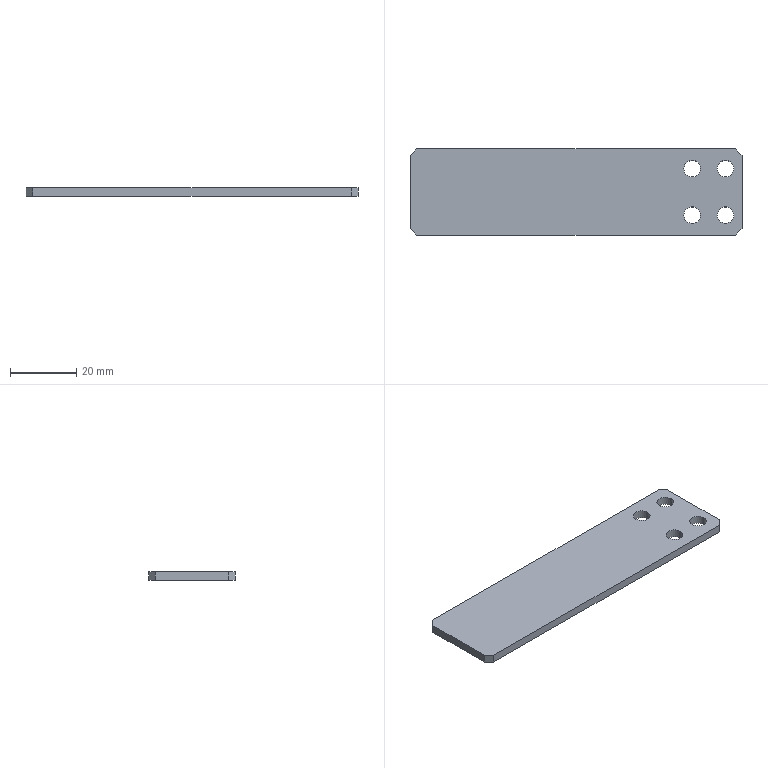Part | STEP file | 1 solid | 18 faces | box 100 x 26 x 2.5 mm | volume 6284 mm3 | plane 10 | cylinder 8 | commonest cylinder face diameters 5 x8
STEP:
#1=CARTESIAN_POINT('',(0.,0.,0.));
#2=DIRECTION('',(0.,0.,1.));
#3=DIRECTION('',(1.,0.,0.));
#4=AXIS2_PLACEMENT_3D('',#1,#2,#3);
#5=CARTESIAN_POINT('',(47.5,-7.,0.));
#6=VERTEX_POINT('',#5);
#7=CARTESIAN_POINT('',(47.5,-7.,2.5));
#8=VERTEX_POINT('',#7);
#9=CARTESIAN_POINT('',(47.5,-7.,0.));
#10=DIRECTION('',(0.,0.,1.));
#11=VECTOR('',#10,1.);
#12=LINE('',#9,#11);
#13=CARTESIAN_POINT('',(45.,-7.,0.));
#14=DIRECTION('',(0.,0.,1.));
#15=DIRECTION('',(1.,0.,0.));
#16=AXIS2_PLACEMENT_3D('',#13,#14,#15);
#17=CYLINDRICAL_SURFACE('',#16,2.5);
#18=CARTESIAN_POINT('',(6.283,0.));
#19=DIRECTION('',(0.,1.));
#20=VECTOR('',#19,1.);
#21=LINE('',#18,#20);
#22=(GEOMETRIC_REPRESENTATION_CONTEXT(2)PARAMETRIC_REPRESENTATION_CONTEXT()REPRESENTATION_CONTEXT('',''));
#23=DEFINITIONAL_REPRESENTATION('',(#21),#22);
#24=PCURVE('',#17,#23);
#25=CARTESIAN_POINT('',(45.,-7.,0.));
#26=DIRECTION('',(0.,0.,1.));
#27=DIRECTION('',(1.,0.,0.));
#28=AXIS2_PLACEMENT_3D('',#25,#26,#27);
#29=CYLINDRICAL_SURFACE('',#28,2.5);
#30=CARTESIAN_POINT('',(0.,0.));
#31=DIRECTION('',(0.,1.));
#32=VECTOR('',#31,1.);
#33=LINE('',#30,#32);
#34=(GEOMETRIC_REPRESENTATION_CONTEXT(2)PARAMETRIC_REPRESENTATION_CONTEXT()REPRESENTATION_CONTEXT('',''));
#35=DEFINITIONAL_REPRESENTATION('',(#33),#34);
#36=PCURVE('',#29,#35);
#37=SURFACE_CURVE('',#12,(#24,#36),.PCURVE_S1.);
#38=EDGE_CURVE('',#6,#8,#37,.T.);
#39=ORIENTED_EDGE('',*,*,#38,.T.);
#40=CARTESIAN_POINT('',(42.5,-7.,2.5));
#41=VERTEX_POINT('',#40);
#42=CARTESIAN_POINT('',(45.,-7.,2.5));
#43=DIRECTION('',(0.,0.,1.));
#44=DIRECTION('',(1.,0.,0.));
#45=AXIS2_PLACEMENT_3D('',#42,#43,#44);
#46=CIRCLE('',#45,2.5);
#47=CARTESIAN_POINT('',(0.,2.5));
#48=DIRECTION('',(1.,0.));
#49=VECTOR('',#48,1.);
#50=LINE('',#47,#49);
#51=(GEOMETRIC_REPRESENTATION_CONTEXT(2)PARAMETRIC_REPRESENTATION_CONTEXT()REPRESENTATION_CONTEXT('',''));
#52=DEFINITIONAL_REPRESENTATION('',(#50),#51);
#53=PCURVE('',#17,#52);
#54=CARTESIAN_POINT('',(-50.,-13.,2.5));
#55=DIRECTION('',(0.,0.,1.));
#56=DIRECTION('',(1.,0.,0.));
#57=AXIS2_PLACEMENT_3D('',#54,#55,#56);
#58=PLANE('',#57);
#59=CARTESIAN_POINT('',(95.,6.));
#60=DIRECTION('',(1.,0.));
#61=AXIS2_PLACEMENT_2D('',#59,#60);
#62=CIRCLE('',#61,2.5);
#63=(GEOMETRIC_REPRESENTATION_CONTEXT(2)PARAMETRIC_REPRESENTATION_CONTEXT()REPRESENTATION_CONTEXT('',''));
#64=DEFINITIONAL_REPRESENTATION('',(#62),#63);
#65=PCURVE('',#58,#64);
#66=SURFACE_CURVE('',#46,(#53,#65),.PCURVE_S1.);
#67=EDGE_CURVE('',#41,#8,#66,.T.);
#68=ORIENTED_EDGE('',*,*,#67,.F.);
#69=CARTESIAN_POINT('',(42.5,-7.,0.));
#70=VERTEX_POINT('',#69);
#71=CARTESIAN_POINT('',(42.5,-7.,0.));
#72=DIRECTION('',(0.,0.,1.));
#73=VECTOR('',#72,1.);
#74=LINE('',#71,#73);
#75=CARTESIAN_POINT('',(3.142,0.));
#76=DIRECTION('',(0.,1.));
#77=VECTOR('',#76,1.);
#78=LINE('',#75,#77);
#79=(GEOMETRIC_REPRESENTATION_CONTEXT(2)PARAMETRIC_REPRESENTATION_CONTEXT()REPRESENTATION_CONTEXT('',''));
#80=DEFINITIONAL_REPRESENTATION('',(#78),#79);
#81=PCURVE('',#17,#80);
#82=CARTESIAN_POINT('',(3.142,0.));
#83=DIRECTION('',(0.,1.));
#84=VECTOR('',#83,1.);
#85=LINE('',#82,#84);
#86=(GEOMETRIC_REPRESENTATION_CONTEXT(2)PARAMETRIC_REPRESENTATION_CONTEXT()REPRESENTATION_CONTEXT('',''));
#87=DEFINITIONAL_REPRESENTATION('',(#85),#86);
#88=PCURVE('',#29,#87);
#89=SURFACE_CURVE('',#74,(#81,#88),.PCURVE_S1.);
#90=EDGE_CURVE('',#70,#41,#89,.T.);
#91=ORIENTED_EDGE('',*,*,#90,.F.);
#92=CARTESIAN_POINT('',(45.,-7.,0.));
#93=DIRECTION('',(0.,0.,-1.));
#94=DIRECTION('',(1.,0.,0.));
#95=AXIS2_PLACEMENT_3D('',#92,#93,#94);
#96=CIRCLE('',#95,2.5);
#97=CARTESIAN_POINT('',(6.283,0.));
#98=DIRECTION('',(-1.,0.));
#99=VECTOR('',#98,1.);
#100=LINE('',#97,#99);
#101=(GEOMETRIC_REPRESENTATION_CONTEXT(2)PARAMETRIC_REPRESENTATION_CONTEXT()REPRESENTATION_CONTEXT('',''));
#102=DEFINITIONAL_REPRESENTATION('',(#100),#101);
#103=PCURVE('',#17,#102);
#104=CARTESIAN_POINT('',(-50.,-13.,0.));
#105=DIRECTION('',(0.,0.,1.));
#106=DIRECTION('',(1.,0.,0.));
#107=AXIS2_PLACEMENT_3D('',#104,#105,#106);
#108=PLANE('',#107);
#109=CARTESIAN_POINT('',(97.5,6.));
#110=CARTESIAN_POINT('',(97.5,1.67));
#111=CARTESIAN_POINT('',(93.75,3.835));
#112=CARTESIAN_POINT('',(90.,6.));
#113=CARTESIAN_POINT('',(93.75,8.165));
#114=CARTESIAN_POINT('',(97.5,10.33));
#115=CARTESIAN_POINT('',(97.5,6.));
#116=(BOUNDED_CURVE()B_SPLINE_CURVE(2,(#109,#110,#111,#112,#113,#114,#115),.UNSPECIFIED.,.T.,.F.)B_SPLINE_CURVE_WITH_KNOTS((1,2,2,2,2,1),(-2.094,0.,2.094,4.189,6.283,8.378),.UNSPECIFIED.)CURVE()GEOMETRIC_REPRESENTATION_ITEM()RATIONAL_B_SPLINE_CURVE((1.,0.5,1.,0.5,1.,0.5,1.))REPRESENTATION_ITEM(''));
#117=(GEOMETRIC_REPRESENTATION_CONTEXT(2)PARAMETRIC_REPRESENTATION_CONTEXT()REPRESENTATION_CONTEXT('',''));
#118=DEFINITIONAL_REPRESENTATION('',(#116),#117);
#119=PCURVE('',#108,#118);
#120=SURFACE_CURVE('',#96,(#103,#119),.PCURVE_S1.);
#121=EDGE_CURVE('',#6,#70,#120,.T.);
#122=ORIENTED_EDGE('',*,*,#121,.F.);
#123=EDGE_LOOP('',(#39,#68,#91,#122));
#124=FACE_BOUND('',#123,.F.);
#125=ADVANCED_FACE('',(#124),#17,.F.);
#126=CARTESIAN_POINT('',(47.5,7.,0.));
#127=VERTEX_POINT('',#126);
#128=CARTESIAN_POINT('',(47.5,7.,2.5));
#129=VERTEX_POINT('',#128);
#130=CARTESIAN_POINT('',(47.5,7.,0.));
#131=DIRECTION('',(0.,0.,1.));
#132=VECTOR('',#131,1.);
#133=LINE('',#130,#132);
#134=CARTESIAN_POINT('',(45.,7.,0.));
#135=DIRECTION('',(0.,0.,1.));
#136=DIRECTION('',(1.,0.,0.));
#137=AXIS2_PLACEMENT_3D('',#134,#135,#136);
#138=CYLINDRICAL_SURFACE('',#137,2.5);
#139=CARTESIAN_POINT('',(6.283,0.));
#140=DIRECTION('',(0.,1.));
#141=VECTOR('',#140,1.);
#142=LINE('',#139,#141);
#143=(GEOMETRIC_REPRESENTATION_CONTEXT(2)PARAMETRIC_REPRESENTATION_CONTEXT()REPRESENTATION_CONTEXT('',''));
#144=DEFINITIONAL_REPRESENTATION('',(#142),#143);
#145=PCURVE('',#138,#144);
#146=CARTESIAN_POINT('',(45.,7.,0.));
#147=DIRECTION('',(0.,0.,1.));
#148=DIRECTION('',(1.,0.,0.));
#149=AXIS2_PLACEMENT_3D('',#146,#147,#148);
#150=CYLINDRICAL_SURFACE('',#149,2.5);
#151=CARTESIAN_POINT('',(0.,0.));
#152=DIRECTION('',(0.,1.));
#153=VECTOR('',#152,1.);
#154=LINE('',#151,#153);
#155=(GEOMETRIC_REPRESENTATION_CONTEXT(2)PARAMETRIC_REPRESENTATION_CONTEXT()REPRESENTATION_CONTEXT('',''));
#156=DEFINITIONAL_REPRESENTATION('',(#154),#155);
#157=PCURVE('',#150,#156);
#158=SURFACE_CURVE('',#133,(#145,#157),.PCURVE_S1.);
#159=EDGE_CURVE('',#127,#129,#158,.T.);
#160=ORIENTED_EDGE('',*,*,#159,.T.);
#161=CARTESIAN_POINT('',(42.5,7.,2.5));
#162=VERTEX_POINT('',#161);
#163=CARTESIAN_POINT('',(45.,7.,2.5));
#164=DIRECTION('',(0.,0.,-1.));
#165=DIRECTION('',(1.,0.,0.));
#166=AXIS2_PLACEMENT_3D('',#163,#164,#165);
#167=CIRCLE('',#166,2.5);
#168=CARTESIAN_POINT('',(6.283,2.5));
#169=DIRECTION('',(-1.,0.));
#170=VECTOR('',#169,1.);
#171=LINE('',#168,#170);
#172=(GEOMETRIC_REPRESENTATION_CONTEXT(2)PARAMETRIC_REPRESENTATION_CONTEXT()REPRESENTATION_CONTEXT('',''));
#173=DEFINITIONAL_REPRESENTATION('',(#171),#172);
#174=PCURVE('',#138,#173);
#175=CARTESIAN_POINT('',(97.5,20.));
#176=CARTESIAN_POINT('',(97.5,15.67));
#177=CARTESIAN_POINT('',(93.75,17.835));
#178=CARTESIAN_POINT('',(90.,20.));
#179=CARTESIAN_POINT('',(93.75,22.165));
#180=CARTESIAN_POINT('',(97.5,24.33));
#181=CARTESIAN_POINT('',(97.5,20.));
#182=(BOUNDED_CURVE()B_SPLINE_CURVE(2,(#175,#176,#177,#178,#179,#180,#181),.UNSPECIFIED.,.T.,.F.)B_SPLINE_CURVE_WITH_KNOTS((1,2,2,2,2,1),(-2.094,0.,2.094,4.189,6.283,8.378),.UNSPECIFIED.)CURVE()GEOMETRIC_REPRESENTATION_ITEM()RATIONAL_B_SPLINE_CURVE((1.,0.5,1.,0.5,1.,0.5,1.))REPRESENTATION_ITEM(''));
#183=(GEOMETRIC_REPRESENTATION_CONTEXT(2)PARAMETRIC_REPRESENTATION_CONTEXT()REPRESENTATION_CONTEXT('',''));
#184=DEFINITIONAL_REPRESENTATION('',(#182),#183);
#185=PCURVE('',#58,#184);
#186=SURFACE_CURVE('',#167,(#174,#185),.PCURVE_S1.);
#187=EDGE_CURVE('',#129,#162,#186,.T.);
#188=ORIENTED_EDGE('',*,*,#187,.T.);
#189=CARTESIAN_POINT('',(42.5,7.,0.));
#190=VERTEX_POINT('',#189);
#191=CARTESIAN_POINT('',(42.5,7.,0.));
#192=DIRECTION('',(0.,0.,1.));
#193=VECTOR('',#192,1.);
#194=LINE('',#191,#193);
#195=CARTESIAN_POINT('',(3.142,0.));
#196=DIRECTION('',(0.,1.));
#197=VECTOR('',#196,1.);
#198=LINE('',#195,#197);
#199=(GEOMETRIC_REPRESENTATION_CONTEXT(2)PARAMETRIC_REPRESENTATION_CONTEXT()REPRESENTATION_CONTEXT('',''));
#200=DEFINITIONAL_REPRESENTATION('',(#198),#199);
#201=PCURVE('',#138,#200);
#202=CARTESIAN_POINT('',(3.142,0.));
#203=DIRECTION('',(0.,1.));
#204=VECTOR('',#203,1.);
#205=LINE('',#202,#204);
#206=(GEOMETRIC_REPRESENTATION_CONTEXT(2)PARAMETRIC_REPRESENTATION_CONTEXT()REPRESENTATION_CONTEXT('',''));
#207=DEFINITIONAL_REPRESENTATION('',(#205),#206);
#208=PCURVE('',#150,#207);
#209=SURFACE_CURVE('',#194,(#201,#208),.PCURVE_S1.);
#210=EDGE_CURVE('',#190,#162,#209,.T.);
#211=ORIENTED_EDGE('',*,*,#210,.F.);
#212=CARTESIAN_POINT('',(45.,7.,0.));
#213=DIRECTION('',(0.,0.,-1.));
#214=DIRECTION('',(1.,0.,0.));
#215=AXIS2_PLACEMENT_3D('',#212,#213,#214);
#216=CIRCLE('',#215,2.5);
#217=CARTESIAN_POINT('',(6.283,0.));
#218=DIRECTION('',(-1.,0.));
#219=VECTOR('',#218,1.);
#220=LINE('',#217,#219);
#221=(GEOMETRIC_REPRESENTATION_CONTEXT(2)PARAMETRIC_REPRESENTATION_CONTEXT()REPRESENTATION_CONTEXT('',''));
#222=DEFINITIONAL_REPRESENTATION('',(#220),#221);
#223=PCURVE('',#138,#222);
#224=CARTESIAN_POINT('',(97.5,20.));
#225=CARTESIAN_POINT('',(97.5,15.67));
#226=CARTESIAN_POINT('',(93.75,17.835));
#227=CARTESIAN_POINT('',(90.,20.));
#228=CARTESIAN_POINT('',(93.75,22.165));
#229=CARTESIAN_POINT('',(97.5,24.33));
#230=CARTESIAN_POINT('',(97.5,20.));
#231=(BOUNDED_CURVE()B_SPLINE_CURVE(2,(#224,#225,#226,#227,#228,#229,#230),.UNSPECIFIED.,.T.,.F.)B_SPLINE_CURVE_WITH_KNOTS((1,2,2,2,2,1),(-2.094,0.,2.094,4.189,6.283,8.378),.UNSPECIFIED.)CURVE()GEOMETRIC_REPRESENTATION_ITEM()RATIONAL_B_SPLINE_CURVE((1.,0.5,1.,0.5,1.,0.5,1.))REPRESENTATION_ITEM(''));
#232=(GEOMETRIC_REPRESENTATION_CONTEXT(2)PARAMETRIC_REPRESENTATION_CONTEXT()REPRESENTATION_CONTEXT('',''));
#233=DEFINITIONAL_REPRESENTATION('',(#231),#232);
#234=PCURVE('',#108,#233);
#235=SURFACE_CURVE('',#216,(#223,#234),.PCURVE_S1.);
#236=EDGE_CURVE('',#127,#190,#235,.T.);
#237=ORIENTED_EDGE('',*,*,#236,.F.);
#238=EDGE_LOOP('',(#160,#188,#211,#237));
#239=FACE_BOUND('',#238,.F.);
#240=ADVANCED_FACE('',(#239),#138,.F.);
#241=CARTESIAN_POINT('',(37.5,7.,0.));
#242=VERTEX_POINT('',#241);
#243=CARTESIAN_POINT('',(37.5,7.,2.5));
#244=VERTEX_POINT('',#243);
#245=CARTESIAN_POINT('',(37.5,7.,0.));
#246=DIRECTION('',(0.,0.,1.));
#247=VECTOR('',#246,1.);
#248=LINE('',#245,#247);
#249=CARTESIAN_POINT('',(35.,7.,0.));
#250=DIRECTION('',(0.,0.,1.));
#251=DIRECTION('',(1.,0.,0.));
#252=AXIS2_PLACEMENT_3D('',#249,#250,#251);
#253=CYLINDRICAL_SURFACE('',#252,2.5);
#254=CARTESIAN_POINT('',(6.283,0.));
#255=DIRECTION('',(0.,1.));
#256=VECTOR('',#255,1.);
#257=LINE('',#254,#256);
#258=(GEOMETRIC_REPRESENTATION_CONTEXT(2)PARAMETRIC_REPRESENTATION_CONTEXT()REPRESENTATION_CONTEXT('',''));
#259=DEFINITIONAL_REPRESENTATION('',(#257),#258);
#260=PCURVE('',#253,#259);
#261=CARTESIAN_POINT('',(35.,7.,0.));
#262=DIRECTION('',(0.,0.,1.));
#263=DIRECTION('',(1.,0.,0.));
#264=AXIS2_PLACEMENT_3D('',#261,#262,#263);
#265=CYLINDRICAL_SURFACE('',#264,2.5);
#266=CARTESIAN_POINT('',(0.,0.));
#267=DIRECTION('',(0.,1.));
#268=VECTOR('',#267,1.);
#269=LINE('',#266,#268);
#270=(GEOMETRIC_REPRESENTATION_CONTEXT(2)PARAMETRIC_REPRESENTATION_CONTEXT()REPRESENTATION_CONTEXT('',''));
#271=DEFINITIONAL_REPRESENTATION('',(#269),#270);
#272=PCURVE('',#265,#271);
#273=SURFACE_CURVE('',#248,(#260,#272),.PCURVE_S1.);
#274=EDGE_CURVE('',#242,#244,#273,.T.);
#275=ORIENTED_EDGE('',*,*,#274,.T.);
#276=CARTESIAN_POINT('',(32.5,7.,2.5));
#277=VERTEX_POINT('',#276);
#278=CARTESIAN_POINT('',(35.,7.,2.5));
#279=DIRECTION('',(0.,0.,-1.));
#280=DIRECTION('',(1.,0.,0.));
#281=AXIS2_PLACEMENT_3D('',#278,#279,#280);
#282=CIRCLE('',#281,2.5);
#283=CARTESIAN_POINT('',(6.283,2.5));
#284=DIRECTION('',(-1.,0.));
#285=VECTOR('',#284,1.);
#286=LINE('',#283,#285);
#287=(GEOMETRIC_REPRESENTATION_CONTEXT(2)PARAMETRIC_REPRESENTATION_CONTEXT()REPRESENTATION_CONTEXT('',''));
#288=DEFINITIONAL_REPRESENTATION('',(#286),#287);
#289=PCURVE('',#253,#288);
#290=CARTESIAN_POINT('',(87.5,20.));
#291=CARTESIAN_POINT('',(87.5,15.67));
#292=CARTESIAN_POINT('',(83.75,17.835));
#293=CARTESIAN_POINT('',(80.,20.));
#294=CARTESIAN_POINT('',(83.75,22.165));
#295=CARTESIAN_POINT('',(87.5,24.33));
#296=CARTESIAN_POINT('',(87.5,20.));
#297=(BOUNDED_CURVE()B_SPLINE_CURVE(2,(#290,#291,#292,#293,#294,#295,#296),.UNSPECIFIED.,.T.,.F.)B_SPLINE_CURVE_WITH_KNOTS((1,2,2,2,2,1),(-2.094,0.,2.094,4.189,6.283,8.378),.UNSPECIFIED.)CURVE()GEOMETRIC_REPRESENTATION_ITEM()RATIONAL_B_SPLINE_CURVE((1.,0.5,1.,0.5,1.,0.5,1.))REPRESENTATION_ITEM(''));
#298=(GEOMETRIC_REPRESENTATION_CONTEXT(2)PARAMETRIC_REPRESENTATION_CONTEXT()REPRESENTATION_CONTEXT('',''));
#299=DEFINITIONAL_REPRESENTATION('',(#297),#298);
#300=PCURVE('',#58,#299);
#301=SURFACE_CURVE('',#282,(#289,#300),.PCURVE_S1.);
#302=EDGE_CURVE('',#244,#277,#301,.T.);
#303=ORIENTED_EDGE('',*,*,#302,.T.);
#304=CARTESIAN_POINT('',(32.5,7.,0.));
#305=VERTEX_POINT('',#304);
#306=CARTESIAN_POINT('',(32.5,7.,0.));
#307=DIRECTION('',(0.,0.,1.));
#308=VECTOR('',#307,1.);
#309=LINE('',#306,#308);
#310=CARTESIAN_POINT('',(3.142,0.));
#311=DIRECTION('',(0.,1.));
#312=VECTOR('',#311,1.);
#313=LINE('',#310,#312);
#314=(GEOMETRIC_REPRESENTATION_CONTEXT(2)PARAMETRIC_REPRESENTATION_CONTEXT()REPRESENTATION_CONTEXT('',''));
#315=DEFINITIONAL_REPRESENTATION('',(#313),#314);
#316=PCURVE('',#253,#315);
#317=CARTESIAN_POINT('',(3.142,0.));
#318=DIRECTION('',(0.,1.));
#319=VECTOR('',#318,1.);
#320=LINE('',#317,#319);
#321=(GEOMETRIC_REPRESENTATION_CONTEXT(2)PARAMETRIC_REPRESENTATION_CONTEXT()REPRESENTATION_CONTEXT('',''));
#322=DEFINITIONAL_REPRESENTATION('',(#320),#321);
#323=PCURVE('',#265,#322);
#324=SURFACE_CURVE('',#309,(#316,#323),.PCURVE_S1.);
#325=EDGE_CURVE('',#305,#277,#324,.T.);
#326=ORIENTED_EDGE('',*,*,#325,.F.);
#327=CARTESIAN_POINT('',(35.,7.,0.));
#328=DIRECTION('',(0.,0.,-1.));
#329=DIRECTION('',(1.,0.,0.));
#330=AXIS2_PLACEMENT_3D('',#327,#328,#329);
#331=CIRCLE('',#330,2.5);
#332=CARTESIAN_POINT('',(6.283,0.));
#333=DIRECTION('',(-1.,0.));
#334=VECTOR('',#333,1.);
#335=LINE('',#332,#334);
#336=(GEOMETRIC_REPRESENTATION_CONTEXT(2)PARAMETRIC_REPRESENTATION_CONTEXT()REPRESENTATION_CONTEXT('',''));
#337=DEFINITIONAL_REPRESENTATION('',(#335),#336);
#338=PCURVE('',#253,#337);
#339=CARTESIAN_POINT('',(87.5,20.));
#340=CARTESIAN_POINT('',(87.5,15.67));
#341=CARTESIAN_POINT('',(83.75,17.835));
#342=CARTESIAN_POINT('',(80.,20.));
#343=CARTESIAN_POINT('',(83.75,22.165));
#344=CARTESIAN_POINT('',(87.5,24.33));
#345=CARTESIAN_POINT('',(87.5,20.));
#346=(BOUNDED_CURVE()B_SPLINE_CURVE(2,(#339,#340,#341,#342,#343,#344,#345),.UNSPECIFIED.,.T.,.F.)B_SPLINE_CURVE_WITH_KNOTS((1,2,2,2,2,1),(-2.094,0.,2.094,4.189,6.283,8.378),.UNSPECIFIED.)CURVE()GEOMETRIC_REPRESENTATION_ITEM()RATIONAL_B_SPLINE_CURVE((1.,0.5,1.,0.5,1.,0.5,1.))REPRESENTATION_ITEM(''));
#347=(GEOMETRIC_REPRESENTATION_CONTEXT(2)PARAMETRIC_REPRESENTATION_CONTEXT()REPRESENTATION_CONTEXT('',''));
#348=DEFINITIONAL_REPRESENTATION('',(#346),#347);
#349=PCURVE('',#108,#348);
#350=SURFACE_CURVE('',#331,(#338,#349),.PCURVE_S1.);
#351=EDGE_CURVE('',#242,#305,#350,.T.);
#352=ORIENTED_EDGE('',*,*,#351,.F.);
#353=EDGE_LOOP('',(#275,#303,#326,#352));
#354=FACE_BOUND('',#353,.F.);
#355=ADVANCED_FACE('',(#354),#253,.F.);
#356=CARTESIAN_POINT('',(37.5,-7.,0.));
#357=VERTEX_POINT('',#356);
#358=CARTESIAN_POINT('',(37.5,-7.,2.5));
#359=VERTEX_POINT('',#358);
#360=CARTESIAN_POINT('',(37.5,-7.,0.));
#361=DIRECTION('',(0.,0.,1.));
#362=VECTOR('',#361,1.);
#363=LINE('',#360,#362);
#364=CARTESIAN_POINT('',(35.,-7.,0.));
#365=DIRECTION('',(0.,0.,1.));
#366=DIRECTION('',(1.,0.,0.));
#367=AXIS2_PLACEMENT_3D('',#364,#365,#366);
#368=CYLINDRICAL_SURFACE('',#367,2.5);
#369=CARTESIAN_POINT('',(6.283,0.));
#370=DIRECTION('',(0.,1.));
#371=VECTOR('',#370,1.);
#372=LINE('',#369,#371);
#373=(GEOMETRIC_REPRESENTATION_CONTEXT(2)PARAMETRIC_REPRESENTATION_CONTEXT()REPRESENTATION_CONTEXT('',''));
#374=DEFINITIONAL_REPRESENTATION('',(#372),#373);
#375=PCURVE('',#368,#374);
#376=CARTESIAN_POINT('',(35.,-7.,0.));
#377=DIRECTION('',(0.,0.,1.));
#378=DIRECTION('',(1.,0.,0.));
#379=AXIS2_PLACEMENT_3D('',#376,#377,#378);
#380=CYLINDRICAL_SURFACE('',#379,2.5);
#381=CARTESIAN_POINT('',(0.,0.));
#382=DIRECTION('',(0.,1.));
#383=VECTOR('',#382,1.);
#384=LINE('',#381,#383);
#385=(GEOMETRIC_REPRESENTATION_CONTEXT(2)PARAMETRIC_REPRESENTATION_CONTEXT()REPRESENTATION_CONTEXT('',''));
#386=DEFINITIONAL_REPRESENTATION('',(#384),#385);
#387=PCURVE('',#380,#386);
#388=SURFACE_CURVE('',#363,(#375,#387),.PCURVE_S1.);
#389=EDGE_CURVE('',#357,#359,#388,.T.);
#390=ORIENTED_EDGE('',*,*,#389,.T.);
#391=CARTESIAN_POINT('',(32.5,-7.,2.5));
#392=VERTEX_POINT('',#391);
#393=CARTESIAN_POINT('',(35.,-7.,2.5));
#394=DIRECTION('',(0.,0.,-1.));
#395=DIRECTION('',(1.,0.,0.));
#396=AXIS2_PLACEMENT_3D('',#393,#394,#395);
#397=CIRCLE('',#396,2.5);
#398=CARTESIAN_POINT('',(6.283,2.5));
#399=DIRECTION('',(-1.,0.));
#400=VECTOR('',#399,1.);
#401=LINE('',#398,#400);
#402=(GEOMETRIC_REPRESENTATION_CONTEXT(2)PARAMETRIC_REPRESENTATION_CONTEXT()REPRESENTATION_CONTEXT('',''));
#403=DEFINITIONAL_REPRESENTATION('',(#401),#402);
#404=PCURVE('',#368,#403);
#405=CARTESIAN_POINT('',(87.5,6.));
#406=CARTESIAN_POINT('',(87.5,1.67));
#407=CARTESIAN_POINT('',(83.75,3.835));
#408=CARTESIAN_POINT('',(80.,6.));
#409=CARTESIAN_POINT('',(83.75,8.165));
#410=CARTESIAN_POINT('',(87.5,10.33));
#411=CARTESIAN_POINT('',(87.5,6.));
#412=(BOUNDED_CURVE()B_SPLINE_CURVE(2,(#405,#406,#407,#408,#409,#410,#411),.UNSPECIFIED.,.T.,.F.)B_SPLINE_CURVE_WITH_KNOTS((1,2,2,2,2,1),(-2.094,0.,2.094,4.189,6.283,8.378),.UNSPECIFIED.)CURVE()GEOMETRIC_REPRESENTATION_ITEM()RATIONAL_B_SPLINE_CURVE((1.,0.5,1.,0.5,1.,0.5,1.))REPRESENTATION_ITEM(''));
#413=(GEOMETRIC_REPRESENTATION_CONTEXT(2)PARAMETRIC_REPRESENTATION_CONTEXT()REPRESENTATION_CONTEXT('',''));
#414=DEFINITIONAL_REPRESENTATION('',(#412),#413);
#415=PCURVE('',#58,#414);
#416=SURFACE_CURVE('',#397,(#404,#415),.PCURVE_S1.);
#417=EDGE_CURVE('',#359,#392,#416,.T.);
#418=ORIENTED_EDGE('',*,*,#417,.T.);
#419=CARTESIAN_POINT('',(32.5,-7.,0.));
#420=VERTEX_POINT('',#419);
#421=CARTESIAN_POINT('',(32.5,-7.,0.));
#422=DIRECTION('',(0.,0.,1.));
#423=VECTOR('',#422,1.);
#424=LINE('',#421,#423);
#425=CARTESIAN_POINT('',(3.142,0.));
#426=DIRECTION('',(0.,1.));
#427=VECTOR('',#426,1.);
#428=LINE('',#425,#427);
#429=(GEOMETRIC_REPRESENTATION_CONTEXT(2)PARAMETRIC_REPRESENTATION_CONTEXT()REPRESENTATION_CONTEXT('',''));
#430=DEFINITIONAL_REPRESENTATION('',(#428),#429);
#431=PCURVE('',#368,#430);
#432=CARTESIAN_POINT('',(3.142,0.));
#433=DIRECTION('',(0.,1.));
#434=VECTOR('',#433,1.);
#435=LINE('',#432,#434);
#436=(GEOMETRIC_REPRESENTATION_CONTEXT(2)PARAMETRIC_REPRESENTATION_CONTEXT()REPRESENTATION_CONTEXT('',''));
#437=DEFINITIONAL_REPRESENTATION('',(#435),#436);
#438=PCURVE('',#380,#437);
#439=SURFACE_CURVE('',#424,(#431,#438),.PCURVE_S1.);
#440=EDGE_CURVE('',#420,#392,#439,.T.);
#441=ORIENTED_EDGE('',*,*,#440,.F.);
#442=CARTESIAN_POINT('',(35.,-7.,0.));
#443=DIRECTION('',(0.,0.,-1.));
#444=DIRECTION('',(1.,0.,0.));
#445=AXIS2_PLACEMENT_3D('',#442,#443,#444);
#446=CIRCLE('',#445,2.5);
#447=CARTESIAN_POINT('',(6.283,0.));
#448=DIRECTION('',(-1.,0.));
#449=VECTOR('',#448,1.);
#450=LINE('',#447,#449);
#451=(GEOMETRIC_REPRESENTATION_CONTEXT(2)PARAMETRIC_REPRESENTATION_CONTEXT()REPRESENTATION_CONTEXT('',''));
#452=DEFINITIONAL_REPRESENTATION('',(#450),#451);
#453=PCURVE('',#368,#452);
#454=CARTESIAN_POINT('',(87.5,6.));
#455=CARTESIAN_POINT('',(87.5,1.67));
#456=CARTESIAN_POINT('',(83.75,3.835));
#457=CARTESIAN_POINT('',(80.,6.));
#458=CARTESIAN_POINT('',(83.75,8.165));
#459=CARTESIAN_POINT('',(87.5,10.33));
#460=CARTESIAN_POINT('',(87.5,6.));
#461=(BOUNDED_CURVE()B_SPLINE_CURVE(2,(#454,#455,#456,#457,#458,#459,#460),.UNSPECIFIED.,.T.,.F.)B_SPLINE_CURVE_WITH_KNOTS((1,2,2,2,2,1),(-2.094,0.,2.094,4.189,6.283,8.378),.UNSPECIFIED.)CURVE()GEOMETRIC_REPRESENTATION_ITEM()RATIONAL_B_SPLINE_CURVE((1.,0.5,1.,0.5,1.,0.5,1.))REPRESENTATION_ITEM(''));
#462=(GEOMETRIC_REPRESENTATION_CONTEXT(2)PARAMETRIC_REPRESENTATION_CONTEXT()REPRESENTATION_CONTEXT('',''));
#463=DEFINITIONAL_REPRESENTATION('',(#461),#462);
#464=PCURVE('',#108,#463);
#465=SURFACE_CURVE('',#446,(#453,#464),.PCURVE_S1.);
#466=EDGE_CURVE('',#357,#420,#465,.T.);
#467=ORIENTED_EDGE('',*,*,#466,.F.);
#468=EDGE_LOOP('',(#390,#418,#441,#467));
#469=FACE_BOUND('',#468,.F.);
#470=ADVANCED_FACE('',(#469),#368,.F.);
#471=CARTESIAN_POINT('',(45.,-7.,2.5));
#472=DIRECTION('',(0.,0.,1.));
#473=DIRECTION('',(1.,0.,0.));
#474=AXIS2_PLACEMENT_3D('',#471,#472,#473);
#475=CIRCLE('',#474,2.5);
#476=CARTESIAN_POINT('',(0.,2.5));
#477=DIRECTION('',(1.,0.));
#478=VECTOR('',#477,1.);
#479=LINE('',#476,#478);
#480=(GEOMETRIC_REPRESENTATION_CONTEXT(2)PARAMETRIC_REPRESENTATION_CONTEXT()REPRESENTATION_CONTEXT('',''));
#481=DEFINITIONAL_REPRESENTATION('',(#479),#480);
#482=PCURVE('',#29,#481);
#483=CARTESIAN_POINT('',(95.,6.));
#484=DIRECTION('',(1.,0.));
#485=AXIS2_PLACEMENT_2D('',#483,#484);
#486=CIRCLE('',#485,2.5);
#487=(GEOMETRIC_REPRESENTATION_CONTEXT(2)PARAMETRIC_REPRESENTATION_CONTEXT()REPRESENTATION_CONTEXT('',''));
#488=DEFINITIONAL_REPRESENTATION('',(#486),#487);
#489=PCURVE('',#58,#488);
#490=SURFACE_CURVE('',#475,(#482,#489),.PCURVE_S1.);
#491=EDGE_CURVE('',#8,#41,#490,.T.);
#492=ORIENTED_EDGE('',*,*,#491,.F.);
#493=ORIENTED_EDGE('',*,*,#38,.F.);
#494=CARTESIAN_POINT('',(45.,-7.,0.));
#495=DIRECTION('',(0.,0.,-1.));
#496=DIRECTION('',(1.,0.,0.));
#497=AXIS2_PLACEMENT_3D('',#494,#495,#496);
#498=CIRCLE('',#497,2.5);
#499=CARTESIAN_POINT('',(6.283,0.));
#500=DIRECTION('',(-1.,0.));
#501=VECTOR('',#500,1.);
#502=LINE('',#499,#501);
#503=(GEOMETRIC_REPRESENTATION_CONTEXT(2)PARAMETRIC_REPRESENTATION_CONTEXT()REPRESENTATION_CONTEXT('',''));
#504=DEFINITIONAL_REPRESENTATION('',(#502),#503);
#505=PCURVE('',#29,#504);
#506=CARTESIAN_POINT('',(97.5,6.));
#507=CARTESIAN_POINT('',(97.5,1.67));
#508=CARTESIAN_POINT('',(93.75,3.835));
#509=CARTESIAN_POINT('',(90.,6.));
#510=CARTESIAN_POINT('',(93.75,8.165));
#511=CARTESIAN_POINT('',(97.5,10.33));
#512=CARTESIAN_POINT('',(97.5,6.));
#513=(BOUNDED_CURVE()B_SPLINE_CURVE(2,(#506,#507,#508,#509,#510,#511,#512),.UNSPECIFIED.,.T.,.F.)B_SPLINE_CURVE_WITH_KNOTS((1,2,2,2,2,1),(-2.094,0.,2.094,4.189,6.283,8.378),.UNSPECIFIED.)CURVE()GEOMETRIC_REPRESENTATION_ITEM()RATIONAL_B_SPLINE_CURVE((1.,0.5,1.,0.5,1.,0.5,1.))REPRESENTATION_ITEM(''));
#514=(GEOMETRIC_REPRESENTATION_CONTEXT(2)PARAMETRIC_REPRESENTATION_CONTEXT()REPRESENTATION_CONTEXT('',''));
#515=DEFINITIONAL_REPRESENTATION('',(#513),#514);
#516=PCURVE('',#108,#515);
#517=SURFACE_CURVE('',#498,(#505,#516),.PCURVE_S1.);
#518=EDGE_CURVE('',#70,#6,#517,.T.);
#519=ORIENTED_EDGE('',*,*,#518,.F.);
#520=ORIENTED_EDGE('',*,*,#90,.T.);
#521=EDGE_LOOP('',(#492,#493,#519,#520));
#522=FACE_BOUND('',#521,.F.);
#523=ADVANCED_FACE('',(#522),#29,.F.);
#524=ORIENTED_EDGE('',*,*,#187,.T.);
#525=CARTESIAN_POINT('',(45.,7.,2.5));
#526=DIRECTION('',(0.,0.,-1.));
#527=DIRECTION('',(1.,0.,0.));
#528=AXIS2_PLACEMENT_3D('',#525,#526,#527);
#529=CIRCLE('',#528,2.5);
#530=CARTESIAN_POINT('',(97.5,20.));
#531=CARTESIAN_POINT('',(97.5,15.67));
#532=CARTESIAN_POINT('',(93.75,17.835));
#533=CARTESIAN_POINT('',(90.,20.));
#534=CARTESIAN_POINT('',(93.75,22.165));
#535=CARTESIAN_POINT('',(97.5,24.33));
#536=CARTESIAN_POINT('',(97.5,20.));
#537=(BOUNDED_CURVE()B_SPLINE_CURVE(2,(#530,#531,#532,#533,#534,#535,#536),.UNSPECIFIED.,.T.,.F.)B_SPLINE_CURVE_WITH_KNOTS((1,2,2,2,2,1),(-2.094,0.,2.094,4.189,6.283,8.378),.UNSPECIFIED.)CURVE()GEOMETRIC_REPRESENTATION_ITEM()RATIONAL_B_SPLINE_CURVE((1.,0.5,1.,0.5,1.,0.5,1.))REPRESENTATION_ITEM(''));
#538=(GEOMETRIC_REPRESENTATION_CONTEXT(2)PARAMETRIC_REPRESENTATION_CONTEXT()REPRESENTATION_CONTEXT('',''));
#539=DEFINITIONAL_REPRESENTATION('',(#537),#538);
#540=PCURVE('',#58,#539);
#541=CARTESIAN_POINT('',(6.283,2.5));
#542=DIRECTION('',(-1.,0.));
#543=VECTOR('',#542,1.);
#544=LINE('',#541,#543);
#545=(GEOMETRIC_REPRESENTATION_CONTEXT(2)PARAMETRIC_REPRESENTATION_CONTEXT()REPRESENTATION_CONTEXT('',''));
#546=DEFINITIONAL_REPRESENTATION('',(#544),#545);
#547=PCURVE('',#150,#546);
#548=SURFACE_CURVE('',#529,(#540,#547),.PCURVE_S1.);
#549=EDGE_CURVE('',#162,#129,#548,.T.);
#550=ORIENTED_EDGE('',*,*,#549,.T.);
#551=EDGE_LOOP('',(#524,#550));
#552=FACE_BOUND('',#551,.T.);
#553=ORIENTED_EDGE('',*,*,#302,.T.);
#554=CARTESIAN_POINT('',(35.,7.,2.5));
#555=DIRECTION('',(0.,0.,-1.));
#556=DIRECTION('',(1.,0.,0.));
#557=AXIS2_PLACEMENT_3D('',#554,#555,#556);
#558=CIRCLE('',#557,2.5);
#559=CARTESIAN_POINT('',(87.5,20.));
#560=CARTESIAN_POINT('',(87.5,15.67));
#561=CARTESIAN_POINT('',(83.75,17.835));
#562=CARTESIAN_POINT('',(80.,20.));
#563=CARTESIAN_POINT('',(83.75,22.165));
#564=CARTESIAN_POINT('',(87.5,24.33));
#565=CARTESIAN_POINT('',(87.5,20.));
#566=(BOUNDED_CURVE()B_SPLINE_CURVE(2,(#559,#560,#561,#562,#563,#564,#565),.UNSPECIFIED.,.T.,.F.)B_SPLINE_CURVE_WITH_KNOTS((1,2,2,2,2,1),(-2.094,0.,2.094,4.189,6.283,8.378),.UNSPECIFIED.)CURVE()GEOMETRIC_REPRESENTATION_ITEM()RATIONAL_B_SPLINE_CURVE((1.,0.5,1.,0.5,1.,0.5,1.))REPRESENTATION_ITEM(''));
#567=(GEOMETRIC_REPRESENTATION_CONTEXT(2)PARAMETRIC_REPRESENTATION_CONTEXT()REPRESENTATION_CONTEXT('',''));
#568=DEFINITIONAL_REPRESENTATION('',(#566),#567);
#569=PCURVE('',#58,#568);
#570=CARTESIAN_POINT('',(6.283,2.5));
#571=DIRECTION('',(-1.,0.));
#572=VECTOR('',#571,1.);
#573=LINE('',#570,#572);
#574=(GEOMETRIC_REPRESENTATION_CONTEXT(2)PARAMETRIC_REPRESENTATION_CONTEXT()REPRESENTATION_CONTEXT('',''));
#575=DEFINITIONAL_REPRESENTATION('',(#573),#574);
#576=PCURVE('',#265,#575);
#577=SURFACE_CURVE('',#558,(#569,#576),.PCURVE_S1.);
#578=EDGE_CURVE('',#277,#244,#577,.T.);
#579=ORIENTED_EDGE('',*,*,#578,.T.);
#580=EDGE_LOOP('',(#553,#579));
#581=FACE_BOUND('',#580,.T.);
#582=ORIENTED_EDGE('',*,*,#417,.T.);
#583=CARTESIAN_POINT('',(35.,-7.,2.5));
#584=DIRECTION('',(0.,0.,-1.));
#585=DIRECTION('',(1.,0.,0.));
#586=AXIS2_PLACEMENT_3D('',#583,#584,#585);
#587=CIRCLE('',#586,2.5);
#588=CARTESIAN_POINT('',(87.5,6.));
#589=CARTESIAN_POINT('',(87.5,1.67));
#590=CARTESIAN_POINT('',(83.75,3.835));
#591=CARTESIAN_POINT('',(80.,6.));
#592=CARTESIAN_POINT('',(83.75,8.165));
#593=CARTESIAN_POINT('',(87.5,10.33));
#594=CARTESIAN_POINT('',(87.5,6.));
#595=(BOUNDED_CURVE()B_SPLINE_CURVE(2,(#588,#589,#590,#591,#592,#593,#594),.UNSPECIFIED.,.T.,.F.)B_SPLINE_CURVE_WITH_KNOTS((1,2,2,2,2,1),(-2.094,0.,2.094,4.189,6.283,8.378),.UNSPECIFIED.)CURVE()GEOMETRIC_REPRESENTATION_ITEM()RATIONAL_B_SPLINE_CURVE((1.,0.5,1.,0.5,1.,0.5,1.))REPRESENTATION_ITEM(''));
#596=(GEOMETRIC_REPRESENTATION_CONTEXT(2)PARAMETRIC_REPRESENTATION_CONTEXT()REPRESENTATION_CONTEXT('',''));
#597=DEFINITIONAL_REPRESENTATION('',(#595),#596);
#598=PCURVE('',#58,#597);
#599=CARTESIAN_POINT('',(6.283,2.5));
#600=DIRECTION('',(-1.,0.));
#601=VECTOR('',#600,1.);
#602=LINE('',#599,#601);
#603=(GEOMETRIC_REPRESENTATION_CONTEXT(2)PARAMETRIC_REPRESENTATION_CONTEXT()REPRESENTATION_CONTEXT('',''));
#604=DEFINITIONAL_REPRESENTATION('',(#602),#603);
#605=PCURVE('',#380,#604);
#606=SURFACE_CURVE('',#587,(#598,#605),.PCURVE_S1.);
#607=EDGE_CURVE('',#392,#359,#606,.T.);
#608=ORIENTED_EDGE('',*,*,#607,.T.);
#609=EDGE_LOOP('',(#582,#608));
#610=FACE_BOUND('',#609,.T.);
#611=ORIENTED_EDGE('',*,*,#491,.F.);
#612=ORIENTED_EDGE('',*,*,#67,.F.);
#613=EDGE_LOOP('',(#611,#612));
#614=FACE_BOUND('',#613,.T.);
#615=CARTESIAN_POINT('',(50.,-11.,2.5));
#616=VERTEX_POINT('',#615);
#617=CARTESIAN_POINT('',(50.,11.,2.5));
#618=VERTEX_POINT('',#617);
#619=CARTESIAN_POINT('',(50.,0.,2.5));
#620=DIRECTION('',(0.,1.,0.));
#621=VECTOR('',#620,1.);
#622=LINE('',#619,#621);
#623=CARTESIAN_POINT('',(100.,13.));
#624=DIRECTION('',(0.,1.));
#625=VECTOR('',#624,1.);
#626=LINE('',#623,#625);
#627=(GEOMETRIC_REPRESENTATION_CONTEXT(2)PARAMETRIC_REPRESENTATION_CONTEXT()REPRESENTATION_CONTEXT('',''));
#628=DEFINITIONAL_REPRESENTATION('',(#626),#627);
#629=PCURVE('',#58,#628);
#630=CARTESIAN_POINT('',(50.,-11.,0.));
#631=DIRECTION('',(-1.,0.,0.));
#632=DIRECTION('',(0.,0.,1.));
#633=AXIS2_PLACEMENT_3D('',#630,#631,#632);
#634=PLANE('',#633);
#635=CARTESIAN_POINT('',(2.5,11.));
#636=DIRECTION('',(0.,1.));
#637=VECTOR('',#636,1.);
#638=LINE('',#635,#637);
#639=(GEOMETRIC_REPRESENTATION_CONTEXT(2)PARAMETRIC_REPRESENTATION_CONTEXT()REPRESENTATION_CONTEXT('',''));
#640=DEFINITIONAL_REPRESENTATION('',(#638),#639);
#641=PCURVE('',#634,#640);
#642=SURFACE_CURVE('',#622,(#629,#641),.PCURVE_S1.);
#643=EDGE_CURVE('',#616,#618,#642,.T.);
#644=ORIENTED_EDGE('',*,*,#643,.T.);
#645=CARTESIAN_POINT('',(48.,13.,2.5));
#646=VERTEX_POINT('',#645);
#647=CARTESIAN_POINT('',(50.,11.,2.5));
#648=DIRECTION('',(-0.7071,0.7071,0.));
#649=VECTOR('',#648,1.);
#650=LINE('',#647,#649);
#651=CARTESIAN_POINT('',(100.,24.));
#652=DIRECTION('',(-0.7071,0.7071));
#653=VECTOR('',#652,1.);
#654=LINE('',#651,#653);
#655=(GEOMETRIC_REPRESENTATION_CONTEXT(2)PARAMETRIC_REPRESENTATION_CONTEXT()REPRESENTATION_CONTEXT('',''));
#656=DEFINITIONAL_REPRESENTATION('',(#654),#655);
#657=PCURVE('',#58,#656);
#658=CARTESIAN_POINT('',(48.,13.,2.5));
#659=DIRECTION('',(-0.7071,-0.7071,0.));
#660=DIRECTION('',(0.,0.,-1.));
#661=AXIS2_PLACEMENT_3D('',#658,#659,#660);
#662=PLANE('',#661);
#663=CARTESIAN_POINT('',(0.,2.828));
#664=DIRECTION('',(0.,-1.));
#665=VECTOR('',#664,1.);
#666=LINE('',#663,#665);
#667=(GEOMETRIC_REPRESENTATION_CONTEXT(2)PARAMETRIC_REPRESENTATION_CONTEXT()REPRESENTATION_CONTEXT('',''));
#668=DEFINITIONAL_REPRESENTATION('',(#666),#667);
#669=PCURVE('',#662,#668);
#670=SURFACE_CURVE('',#650,(#657,#669),.PCURVE_S1.);
#671=EDGE_CURVE('',#618,#646,#670,.T.);
#672=ORIENTED_EDGE('',*,*,#671,.T.);
#673=CARTESIAN_POINT('',(-48.,13.,2.5));
#674=VERTEX_POINT('',#673);
#675=CARTESIAN_POINT('',(0.,13.,2.5));
#676=DIRECTION('',(-1.,0.,0.));
#677=VECTOR('',#676,1.);
#678=LINE('',#675,#677);
#679=CARTESIAN_POINT('',(50.,26.));
#680=DIRECTION('',(-1.,0.));
#681=VECTOR('',#680,1.);
#682=LINE('',#679,#681);
#683=(GEOMETRIC_REPRESENTATION_CONTEXT(2)PARAMETRIC_REPRESENTATION_CONTEXT()REPRESENTATION_CONTEXT('',''));
#684=DEFINITIONAL_REPRESENTATION('',(#682),#683);
#685=PCURVE('',#58,#684);
#686=CARTESIAN_POINT('',(-48.,13.,2.5));
#687=DIRECTION('',(0.,-1.,0.));
#688=DIRECTION('',(0.,0.,-1.));
#689=AXIS2_PLACEMENT_3D('',#686,#687,#688);
#690=PLANE('',#689);
#691=CARTESIAN_POINT('',(0.,48.));
#692=DIRECTION('',(0.,-1.));
#693=VECTOR('',#692,1.);
#694=LINE('',#691,#693);
#695=(GEOMETRIC_REPRESENTATION_CONTEXT(2)PARAMETRIC_REPRESENTATION_CONTEXT()REPRESENTATION_CONTEXT('',''));
#696=DEFINITIONAL_REPRESENTATION('',(#694),#695);
#697=PCURVE('',#690,#696);
#698=SURFACE_CURVE('',#678,(#685,#697),.PCURVE_S1.);
#699=EDGE_CURVE('',#646,#674,#698,.T.);
#700=ORIENTED_EDGE('',*,*,#699,.T.);
#701=CARTESIAN_POINT('',(-50.,11.,2.5));
#702=VERTEX_POINT('',#701);
#703=CARTESIAN_POINT('',(-48.,13.,2.5));
#704=DIRECTION('',(-0.7071,-0.7071,0.));
#705=VECTOR('',#704,1.);
#706=LINE('',#703,#705);
#707=CARTESIAN_POINT('',(2.,26.));
#708=DIRECTION('',(-0.7071,-0.7071));
#709=VECTOR('',#708,1.);
#710=LINE('',#707,#709);
#711=(GEOMETRIC_REPRESENTATION_CONTEXT(2)PARAMETRIC_REPRESENTATION_CONTEXT()REPRESENTATION_CONTEXT('',''));
#712=DEFINITIONAL_REPRESENTATION('',(#710),#711);
#713=PCURVE('',#58,#712);
#714=CARTESIAN_POINT('',(-50.,11.,2.5));
#715=DIRECTION('',(0.7071,-0.7071,0.));
#716=DIRECTION('',(0.,0.,-1.));
#717=AXIS2_PLACEMENT_3D('',#714,#715,#716);
#718=PLANE('',#717);
#719=CARTESIAN_POINT('',(0.,2.828));
#720=DIRECTION('',(0.,-1.));
#721=VECTOR('',#720,1.);
#722=LINE('',#719,#721);
#723=(GEOMETRIC_REPRESENTATION_CONTEXT(2)PARAMETRIC_REPRESENTATION_CONTEXT()REPRESENTATION_CONTEXT('',''));
#724=DEFINITIONAL_REPRESENTATION('',(#722),#723);
#725=PCURVE('',#718,#724);
#726=SURFACE_CURVE('',#706,(#713,#725),.PCURVE_S1.);
#727=EDGE_CURVE('',#674,#702,#726,.T.);
#728=ORIENTED_EDGE('',*,*,#727,.T.);
#729=CARTESIAN_POINT('',(-50.,-11.,2.5));
#730=VERTEX_POINT('',#729);
#731=CARTESIAN_POINT('',(-50.,0.,2.5));
#732=DIRECTION('',(0.,-1.,0.));
#733=VECTOR('',#732,1.);
#734=LINE('',#731,#733);
#735=CARTESIAN_POINT('',(0.,13.));
#736=DIRECTION('',(0.,-1.));
#737=VECTOR('',#736,1.);
#738=LINE('',#735,#737);
#739=(GEOMETRIC_REPRESENTATION_CONTEXT(2)PARAMETRIC_REPRESENTATION_CONTEXT()REPRESENTATION_CONTEXT('',''));
#740=DEFINITIONAL_REPRESENTATION('',(#738),#739);
#741=PCURVE('',#58,#740);
#742=CARTESIAN_POINT('',(-50.,-11.,2.5));
#743=DIRECTION('',(1.,0.,0.));
#744=DIRECTION('',(0.,0.,-1.));
#745=AXIS2_PLACEMENT_3D('',#742,#743,#744);
#746=PLANE('',#745);
#747=CARTESIAN_POINT('',(0.,11.));
#748=DIRECTION('',(0.,-1.));
#749=VECTOR('',#748,1.);
#750=LINE('',#747,#749);
#751=(GEOMETRIC_REPRESENTATION_CONTEXT(2)PARAMETRIC_REPRESENTATION_CONTEXT()REPRESENTATION_CONTEXT('',''));
#752=DEFINITIONAL_REPRESENTATION('',(#750),#751);
#753=PCURVE('',#746,#752);
#754=SURFACE_CURVE('',#734,(#741,#753),.PCURVE_S1.);
#755=EDGE_CURVE('',#702,#730,#754,.T.);
#756=ORIENTED_EDGE('',*,*,#755,.T.);
#757=CARTESIAN_POINT('',(-48.,-13.,2.5));
#758=VERTEX_POINT('',#757);
#759=CARTESIAN_POINT('',(-50.,-11.,2.5));
#760=DIRECTION('',(0.7071,-0.7071,0.));
#761=VECTOR('',#760,1.);
#762=LINE('',#759,#761);
#763=CARTESIAN_POINT('',(0.,2.));
#764=DIRECTION('',(0.7071,-0.7071));
#765=VECTOR('',#764,1.);
#766=LINE('',#763,#765);
#767=(GEOMETRIC_REPRESENTATION_CONTEXT(2)PARAMETRIC_REPRESENTATION_CONTEXT()REPRESENTATION_CONTEXT('',''));
#768=DEFINITIONAL_REPRESENTATION('',(#766),#767);
#769=PCURVE('',#58,#768);
#770=CARTESIAN_POINT('',(-48.,-13.,2.5));
#771=DIRECTION('',(0.7071,0.7071,0.));
#772=DIRECTION('',(0.,0.,-1.));
#773=AXIS2_PLACEMENT_3D('',#770,#771,#772);
#774=PLANE('',#773);
#775=CARTESIAN_POINT('',(0.,2.828));
#776=DIRECTION('',(0.,-1.));
#777=VECTOR('',#776,1.);
#778=LINE('',#775,#777);
#779=(GEOMETRIC_REPRESENTATION_CONTEXT(2)PARAMETRIC_REPRESENTATION_CONTEXT()REPRESENTATION_CONTEXT('',''));
#780=DEFINITIONAL_REPRESENTATION('',(#778),#779);
#781=PCURVE('',#774,#780);
#782=SURFACE_CURVE('',#762,(#769,#781),.PCURVE_S1.);
#783=EDGE_CURVE('',#730,#758,#782,.T.);
#784=ORIENTED_EDGE('',*,*,#783,.T.);
#785=CARTESIAN_POINT('',(48.,-13.,2.5));
#786=VERTEX_POINT('',#785);
#787=CARTESIAN_POINT('',(0.,-13.,2.5));
#788=DIRECTION('',(1.,0.,0.));
#789=VECTOR('',#788,1.);
#790=LINE('',#787,#789);
#791=CARTESIAN_POINT('',(50.,0.));
#792=DIRECTION('',(1.,0.));
#793=VECTOR('',#792,1.);
#794=LINE('',#791,#793);
#795=(GEOMETRIC_REPRESENTATION_CONTEXT(2)PARAMETRIC_REPRESENTATION_CONTEXT()REPRESENTATION_CONTEXT('',''));
#796=DEFINITIONAL_REPRESENTATION('',(#794),#795);
#797=PCURVE('',#58,#796);
#798=CARTESIAN_POINT('',(48.,-13.,0.));
#799=DIRECTION('',(0.,1.,0.));
#800=DIRECTION('',(-1.,0.,0.));
#801=AXIS2_PLACEMENT_3D('',#798,#799,#800);
#802=PLANE('',#801);
#803=CARTESIAN_POINT('',(48.,2.5));
#804=DIRECTION('',(-1.,0.));
#805=VECTOR('',#804,1.);
#806=LINE('',#803,#805);
#807=(GEOMETRIC_REPRESENTATION_CONTEXT(2)PARAMETRIC_REPRESENTATION_CONTEXT()REPRESENTATION_CONTEXT('',''));
#808=DEFINITIONAL_REPRESENTATION('',(#806),#807);
#809=PCURVE('',#802,#808);
#810=SURFACE_CURVE('',#790,(#797,#809),.PCURVE_S1.);
#811=EDGE_CURVE('',#758,#786,#810,.T.);
#812=ORIENTED_EDGE('',*,*,#811,.T.);
#813=CARTESIAN_POINT('',(48.,-13.,2.5));
#814=DIRECTION('',(0.7071,0.7071,0.));
#815=VECTOR('',#814,1.);
#816=LINE('',#813,#815);
#817=CARTESIAN_POINT('',(98.,0.));
#818=DIRECTION('',(0.7071,0.7071));
#819=VECTOR('',#818,1.);
#820=LINE('',#817,#819);
#821=(GEOMETRIC_REPRESENTATION_CONTEXT(2)PARAMETRIC_REPRESENTATION_CONTEXT()REPRESENTATION_CONTEXT('',''));
#822=DEFINITIONAL_REPRESENTATION('',(#820),#821);
#823=PCURVE('',#58,#822);
#824=CARTESIAN_POINT('',(50.,-11.,2.5));
#825=DIRECTION('',(-0.7071,0.7071,0.));
#826=DIRECTION('',(0.,0.,-1.));
#827=AXIS2_PLACEMENT_3D('',#824,#825,#826);
#828=PLANE('',#827);
#829=CARTESIAN_POINT('',(0.,2.828));
#830=DIRECTION('',(0.,-1.));
#831=VECTOR('',#830,1.);
#832=LINE('',#829,#831);
#833=(GEOMETRIC_REPRESENTATION_CONTEXT(2)PARAMETRIC_REPRESENTATION_CONTEXT()REPRESENTATION_CONTEXT('',''));
#834=DEFINITIONAL_REPRESENTATION('',(#832),#833);
#835=PCURVE('',#828,#834);
#836=SURFACE_CURVE('',#816,(#823,#835),.PCURVE_S1.);
#837=EDGE_CURVE('',#786,#616,#836,.T.);
#838=ORIENTED_EDGE('',*,*,#837,.T.);
#839=EDGE_LOOP('',(#644,#672,#700,#728,#756,#784,#812,#838));
#840=FACE_BOUND('',#839,.T.);
#841=ADVANCED_FACE('',(#552,#581,#610,#614,#840),#58,.T.);
#842=ORIENTED_EDGE('',*,*,#236,.F.);
#843=CARTESIAN_POINT('',(45.,7.,0.));
#844=DIRECTION('',(0.,0.,-1.));
#845=DIRECTION('',(1.,0.,0.));
#846=AXIS2_PLACEMENT_3D('',#843,#844,#845);
#847=CIRCLE('',#846,2.5);
#848=CARTESIAN_POINT('',(97.5,20.));
#849=CARTESIAN_POINT('',(97.5,15.67));
#850=CARTESIAN_POINT('',(93.75,17.835));
#851=CARTESIAN_POINT('',(90.,20.));
#852=CARTESIAN_POINT('',(93.75,22.165));
#853=CARTESIAN_POINT('',(97.5,24.33));
#854=CARTESIAN_POINT('',(97.5,20.));
#855=(BOUNDED_CURVE()B_SPLINE_CURVE(2,(#848,#849,#850,#851,#852,#853,#854),.UNSPECIFIED.,.T.,.F.)B_SPLINE_CURVE_WITH_KNOTS((1,2,2,2,2,1),(-2.094,0.,2.094,4.189,6.283,8.378),.UNSPECIFIED.)CURVE()GEOMETRIC_REPRESENTATION_ITEM()RATIONAL_B_SPLINE_CURVE((1.,0.5,1.,0.5,1.,0.5,1.))REPRESENTATION_ITEM(''));
#856=(GEOMETRIC_REPRESENTATION_CONTEXT(2)PARAMETRIC_REPRESENTATION_CONTEXT()REPRESENTATION_CONTEXT('',''));
#857=DEFINITIONAL_REPRESENTATION('',(#855),#856);
#858=PCURVE('',#108,#857);
#859=CARTESIAN_POINT('',(6.283,0.));
#860=DIRECTION('',(-1.,0.));
#861=VECTOR('',#860,1.);
#862=LINE('',#859,#861);
#863=(GEOMETRIC_REPRESENTATION_CONTEXT(2)PARAMETRIC_REPRESENTATION_CONTEXT()REPRESENTATION_CONTEXT('',''));
#864=DEFINITIONAL_REPRESENTATION('',(#862),#863);
#865=PCURVE('',#150,#864);
#866=SURFACE_CURVE('',#847,(#858,#865),.PCURVE_S1.);
#867=EDGE_CURVE('',#190,#127,#866,.T.);
#868=ORIENTED_EDGE('',*,*,#867,.F.);
#869=EDGE_LOOP('',(#842,#868));
#870=FACE_BOUND('',#869,.T.);
#871=ORIENTED_EDGE('',*,*,#351,.F.);
#872=CARTESIAN_POINT('',(35.,7.,0.));
#873=DIRECTION('',(0.,0.,-1.));
#874=DIRECTION('',(1.,0.,0.));
#875=AXIS2_PLACEMENT_3D('',#872,#873,#874);
#876=CIRCLE('',#875,2.5);
#877=CARTESIAN_POINT('',(87.5,20.));
#878=CARTESIAN_POINT('',(87.5,15.67));
#879=CARTESIAN_POINT('',(83.75,17.835));
#880=CARTESIAN_POINT('',(80.,20.));
#881=CARTESIAN_POINT('',(83.75,22.165));
#882=CARTESIAN_POINT('',(87.5,24.33));
#883=CARTESIAN_POINT('',(87.5,20.));
#884=(BOUNDED_CURVE()B_SPLINE_CURVE(2,(#877,#878,#879,#880,#881,#882,#883),.UNSPECIFIED.,.T.,.F.)B_SPLINE_CURVE_WITH_KNOTS((1,2,2,2,2,1),(-2.094,0.,2.094,4.189,6.283,8.378),.UNSPECIFIED.)CURVE()GEOMETRIC_REPRESENTATION_ITEM()RATIONAL_B_SPLINE_CURVE((1.,0.5,1.,0.5,1.,0.5,1.))REPRESENTATION_ITEM(''));
#885=(GEOMETRIC_REPRESENTATION_CONTEXT(2)PARAMETRIC_REPRESENTATION_CONTEXT()REPRESENTATION_CONTEXT('',''));
#886=DEFINITIONAL_REPRESENTATION('',(#884),#885);
#887=PCURVE('',#108,#886);
#888=CARTESIAN_POINT('',(6.283,0.));
#889=DIRECTION('',(-1.,0.));
#890=VECTOR('',#889,1.);
#891=LINE('',#888,#890);
#892=(GEOMETRIC_REPRESENTATION_CONTEXT(2)PARAMETRIC_REPRESENTATION_CONTEXT()REPRESENTATION_CONTEXT('',''));
#893=DEFINITIONAL_REPRESENTATION('',(#891),#892);
#894=PCURVE('',#265,#893);
#895=SURFACE_CURVE('',#876,(#887,#894),.PCURVE_S1.);
#896=EDGE_CURVE('',#305,#242,#895,.T.);
#897=ORIENTED_EDGE('',*,*,#896,.F.);
#898=EDGE_LOOP('',(#871,#897));
#899=FACE_BOUND('',#898,.T.);
#900=ORIENTED_EDGE('',*,*,#466,.F.);
#901=CARTESIAN_POINT('',(35.,-7.,0.));
#902=DIRECTION('',(0.,0.,-1.));
#903=DIRECTION('',(1.,0.,0.));
#904=AXIS2_PLACEMENT_3D('',#901,#902,#903);
#905=CIRCLE('',#904,2.5);
#906=CARTESIAN_POINT('',(87.5,6.));
#907=CARTESIAN_POINT('',(87.5,1.67));
#908=CARTESIAN_POINT('',(83.75,3.835));
#909=CARTESIAN_POINT('',(80.,6.));
#910=CARTESIAN_POINT('',(83.75,8.165));
#911=CARTESIAN_POINT('',(87.5,10.33));
#912=CARTESIAN_POINT('',(87.5,6.));
#913=(BOUNDED_CURVE()B_SPLINE_CURVE(2,(#906,#907,#908,#909,#910,#911,#912),.UNSPECIFIED.,.T.,.F.)B_SPLINE_CURVE_WITH_KNOTS((1,2,2,2,2,1),(-2.094,0.,2.094,4.189,6.283,8.378),.UNSPECIFIED.)CURVE()GEOMETRIC_REPRESENTATION_ITEM()RATIONAL_B_SPLINE_CURVE((1.,0.5,1.,0.5,1.,0.5,1.))REPRESENTATION_ITEM(''));
#914=(GEOMETRIC_REPRESENTATION_CONTEXT(2)PARAMETRIC_REPRESENTATION_CONTEXT()REPRESENTATION_CONTEXT('',''));
#915=DEFINITIONAL_REPRESENTATION('',(#913),#914);
#916=PCURVE('',#108,#915);
#917=CARTESIAN_POINT('',(6.283,0.));
#918=DIRECTION('',(-1.,0.));
#919=VECTOR('',#918,1.);
#920=LINE('',#917,#919);
#921=(GEOMETRIC_REPRESENTATION_CONTEXT(2)PARAMETRIC_REPRESENTATION_CONTEXT()REPRESENTATION_CONTEXT('',''));
#922=DEFINITIONAL_REPRESENTATION('',(#920),#921);
#923=PCURVE('',#380,#922);
#924=SURFACE_CURVE('',#905,(#916,#923),.PCURVE_S1.);
#925=EDGE_CURVE('',#420,#357,#924,.T.);
#926=ORIENTED_EDGE('',*,*,#925,.F.);
#927=EDGE_LOOP('',(#900,#926));
#928=FACE_BOUND('',#927,.T.);
#929=ORIENTED_EDGE('',*,*,#121,.F.);
#930=ORIENTED_EDGE('',*,*,#518,.F.);
#931=EDGE_LOOP('',(#929,#930));
#932=FACE_BOUND('',#931,.T.);
#933=CARTESIAN_POINT('',(-48.,13.,0.));
#934=VERTEX_POINT('',#933);
#935=CARTESIAN_POINT('',(-50.,11.,0.));
#936=VERTEX_POINT('',#935);
#937=CARTESIAN_POINT('',(-50.,11.,0.));
#938=DIRECTION('',(-0.7071,-0.7071,0.));
#939=VECTOR('',#938,1.);
#940=LINE('',#937,#939);
#941=CARTESIAN_POINT('',(0.,24.));
#942=DIRECTION('',(-0.7071,-0.7071));
#943=VECTOR('',#942,1.);
#944=LINE('',#941,#943);
#945=(GEOMETRIC_REPRESENTATION_CONTEXT(2)PARAMETRIC_REPRESENTATION_CONTEXT()REPRESENTATION_CONTEXT('',''));
#946=DEFINITIONAL_REPRESENTATION('',(#944),#945);
#947=PCURVE('',#108,#946);
#948=CARTESIAN_POINT('',(2.5,0.));
#949=DIRECTION('',(0.,-1.));
#950=VECTOR('',#949,1.);
#951=LINE('',#948,#950);
#952=(GEOMETRIC_REPRESENTATION_CONTEXT(2)PARAMETRIC_REPRESENTATION_CONTEXT()REPRESENTATION_CONTEXT('',''));
#953=DEFINITIONAL_REPRESENTATION('',(#951),#952);
#954=PCURVE('',#718,#953);
#955=SURFACE_CURVE('',#940,(#947,#954),.PCURVE_S1.);
#956=EDGE_CURVE('',#934,#936,#955,.T.);
#957=ORIENTED_EDGE('',*,*,#956,.F.);
#958=CARTESIAN_POINT('',(48.,13.,0.));
#959=VERTEX_POINT('',#958);
#960=CARTESIAN_POINT('',(0.,13.,0.));
#961=DIRECTION('',(-1.,0.,0.));
#962=VECTOR('',#961,1.);
#963=LINE('',#960,#962);
#964=CARTESIAN_POINT('',(50.,26.));
#965=DIRECTION('',(-1.,0.));
#966=VECTOR('',#965,1.);
#967=LINE('',#964,#966);
#968=(GEOMETRIC_REPRESENTATION_CONTEXT(2)PARAMETRIC_REPRESENTATION_CONTEXT()REPRESENTATION_CONTEXT('',''));
#969=DEFINITIONAL_REPRESENTATION('',(#967),#968);
#970=PCURVE('',#108,#969);
#971=CARTESIAN_POINT('',(2.5,48.));
#972=DIRECTION('',(0.,-1.));
#973=VECTOR('',#972,1.);
#974=LINE('',#971,#973);
#975=(GEOMETRIC_REPRESENTATION_CONTEXT(2)PARAMETRIC_REPRESENTATION_CONTEXT()REPRESENTATION_CONTEXT('',''));
#976=DEFINITIONAL_REPRESENTATION('',(#974),#975);
#977=PCURVE('',#690,#976);
#978=SURFACE_CURVE('',#963,(#970,#977),.PCURVE_S1.);
#979=EDGE_CURVE('',#959,#934,#978,.T.);
#980=ORIENTED_EDGE('',*,*,#979,.F.);
#981=CARTESIAN_POINT('',(50.,11.,0.));
#982=VERTEX_POINT('',#981);
#983=CARTESIAN_POINT('',(48.,13.,0.));
#984=DIRECTION('',(-0.7071,0.7071,0.));
#985=VECTOR('',#984,1.);
#986=LINE('',#983,#985);
#987=CARTESIAN_POINT('',(98.,26.));
#988=DIRECTION('',(-0.7071,0.7071));
#989=VECTOR('',#988,1.);
#990=LINE('',#987,#989);
#991=(GEOMETRIC_REPRESENTATION_CONTEXT(2)PARAMETRIC_REPRESENTATION_CONTEXT()REPRESENTATION_CONTEXT('',''));
#992=DEFINITIONAL_REPRESENTATION('',(#990),#991);
#993=PCURVE('',#108,#992);
#994=CARTESIAN_POINT('',(2.5,0.));
#995=DIRECTION('',(0.,-1.));
#996=VECTOR('',#995,1.);
#997=LINE('',#994,#996);
#998=(GEOMETRIC_REPRESENTATION_CONTEXT(2)PARAMETRIC_REPRESENTATION_CONTEXT()REPRESENTATION_CONTEXT('',''));
#999=DEFINITIONAL_REPRESENTATION('',(#997),#998);
#1000=PCURVE('',#662,#999);
#1001=SURFACE_CURVE('',#986,(#993,#1000),.PCURVE_S1.);
#1002=EDGE_CURVE('',#982,#959,#1001,.T.);
#1003=ORIENTED_EDGE('',*,*,#1002,.F.);
#1004=CARTESIAN_POINT('',(50.,-11.,0.));
#1005=VERTEX_POINT('',#1004);
#1006=CARTESIAN_POINT('',(50.,0.,0.));
#1007=DIRECTION('',(0.,1.,0.));
#1008=VECTOR('',#1007,1.);
#1009=LINE('',#1006,#1008);
#1010=CARTESIAN_POINT('',(100.,13.));
#1011=DIRECTION('',(0.,1.));
#1012=VECTOR('',#1011,1.);
#1013=LINE('',#1010,#1012);
#1014=(GEOMETRIC_REPRESENTATION_CONTEXT(2)PARAMETRIC_REPRESENTATION_CONTEXT()REPRESENTATION_CONTEXT('',''));
#1015=DEFINITIONAL_REPRESENTATION('',(#1013),#1014);
#1016=PCURVE('',#108,#1015);
#1017=CARTESIAN_POINT('',(0.,11.));
#1018=DIRECTION('',(0.,1.));
#1019=VECTOR('',#1018,1.);
#1020=LINE('',#1017,#1019);
#1021=(GEOMETRIC_REPRESENTATION_CONTEXT(2)PARAMETRIC_REPRESENTATION_CONTEXT()REPRESENTATION_CONTEXT('',''));
#1022=DEFINITIONAL_REPRESENTATION('',(#1020),#1021);
#1023=PCURVE('',#634,#1022);
#1024=SURFACE_CURVE('',#1009,(#1016,#1023),.PCURVE_S1.);
#1025=EDGE_CURVE('',#1005,#982,#1024,.T.);
#1026=ORIENTED_EDGE('',*,*,#1025,.F.);
#1027=CARTESIAN_POINT('',(48.,-13.,0.));
#1028=VERTEX_POINT('',#1027);
#1029=CARTESIAN_POINT('',(50.,-11.,0.));
#1030=DIRECTION('',(0.7071,0.7071,0.));
#1031=VECTOR('',#1030,1.);
#1032=LINE('',#1029,#1031);
#1033=CARTESIAN_POINT('',(100.,2.));
#1034=DIRECTION('',(0.7071,0.7071));
#1035=VECTOR('',#1034,1.);
#1036=LINE('',#1033,#1035);
#1037=(GEOMETRIC_REPRESENTATION_CONTEXT(2)PARAMETRIC_REPRESENTATION_CONTEXT()REPRESENTATION_CONTEXT('',''));
#1038=DEFINITIONAL_REPRESENTATION('',(#1036),#1037);
#1039=PCURVE('',#108,#1038);
#1040=CARTESIAN_POINT('',(2.5,0.));
#1041=DIRECTION('',(0.,-1.));
#1042=VECTOR('',#1041,1.);
#1043=LINE('',#1040,#1042);
#1044=(GEOMETRIC_REPRESENTATION_CONTEXT(2)PARAMETRIC_REPRESENTATION_CONTEXT()REPRESENTATION_CONTEXT('',''));
#1045=DEFINITIONAL_REPRESENTATION('',(#1043),#1044);
#1046=PCURVE('',#828,#1045);
#1047=SURFACE_CURVE('',#1032,(#1039,#1046),.PCURVE_S1.);
#1048=EDGE_CURVE('',#1028,#1005,#1047,.T.);
#1049=ORIENTED_EDGE('',*,*,#1048,.F.);
#1050=CARTESIAN_POINT('',(-48.,-13.,0.));
#1051=VERTEX_POINT('',#1050);
#1052=CARTESIAN_POINT('',(0.,-13.,0.));
#1053=DIRECTION('',(1.,0.,0.));
#1054=VECTOR('',#1053,1.);
#1055=LINE('',#1052,#1054);
#1056=CARTESIAN_POINT('',(50.,0.));
#1057=DIRECTION('',(1.,0.));
#1058=VECTOR('',#1057,1.);
#1059=LINE('',#1056,#1058);
#1060=(GEOMETRIC_REPRESENTATION_CONTEXT(2)PARAMETRIC_REPRESENTATION_CONTEXT()REPRESENTATION_CONTEXT('',''));
#1061=DEFINITIONAL_REPRESENTATION('',(#1059),#1060);
#1062=PCURVE('',#108,#1061);
#1063=CARTESIAN_POINT('',(48.,0.));
#1064=DIRECTION('',(-1.,0.));
#1065=VECTOR('',#1064,1.);
#1066=LINE('',#1063,#1065);
#1067=(GEOMETRIC_REPRESENTATION_CONTEXT(2)PARAMETRIC_REPRESENTATION_CONTEXT()REPRESENTATION_CONTEXT('',''));
#1068=DEFINITIONAL_REPRESENTATION('',(#1066),#1067);
#1069=PCURVE('',#802,#1068);
#1070=SURFACE_CURVE('',#1055,(#1062,#1069),.PCURVE_S1.);
#1071=EDGE_CURVE('',#1051,#1028,#1070,.T.);
#1072=ORIENTED_EDGE('',*,*,#1071,.F.);
#1073=CARTESIAN_POINT('',(-50.,-11.,0.));
#1074=VERTEX_POINT('',#1073);
#1075=CARTESIAN_POINT('',(-48.,-13.,0.));
#1076=DIRECTION('',(0.7071,-0.7071,0.));
#1077=VECTOR('',#1076,1.);
#1078=LINE('',#1075,#1077);
#1079=CARTESIAN_POINT('',(2.,0.));
#1080=DIRECTION('',(0.7071,-0.7071));
#1081=VECTOR('',#1080,1.);
#1082=LINE('',#1079,#1081);
#1083=(GEOMETRIC_REPRESENTATION_CONTEXT(2)PARAMETRIC_REPRESENTATION_CONTEXT()REPRESENTATION_CONTEXT('',''));
#1084=DEFINITIONAL_REPRESENTATION('',(#1082),#1083);
#1085=PCURVE('',#108,#1084);
#1086=CARTESIAN_POINT('',(2.5,0.));
#1087=DIRECTION('',(0.,-1.));
#1088=VECTOR('',#1087,1.);
#1089=LINE('',#1086,#1088);
#1090=(GEOMETRIC_REPRESENTATION_CONTEXT(2)PARAMETRIC_REPRESENTATION_CONTEXT()REPRESENTATION_CONTEXT('',''));
#1091=DEFINITIONAL_REPRESENTATION('',(#1089),#1090);
#1092=PCURVE('',#774,#1091);
#1093=SURFACE_CURVE('',#1078,(#1085,#1092),.PCURVE_S1.);
#1094=EDGE_CURVE('',#1074,#1051,#1093,.T.);
#1095=ORIENTED_EDGE('',*,*,#1094,.F.);
#1096=CARTESIAN_POINT('',(-50.,0.,0.));
#1097=DIRECTION('',(0.,-1.,0.));
#1098=VECTOR('',#1097,1.);
#1099=LINE('',#1096,#1098);
#1100=CARTESIAN_POINT('',(0.,13.));
#1101=DIRECTION('',(0.,-1.));
#1102=VECTOR('',#1101,1.);
#1103=LINE('',#1100,#1102);
#1104=(GEOMETRIC_REPRESENTATION_CONTEXT(2)PARAMETRIC_REPRESENTATION_CONTEXT()REPRESENTATION_CONTEXT('',''));
#1105=DEFINITIONAL_REPRESENTATION('',(#1103),#1104);
#1106=PCURVE('',#108,#1105);
#1107=CARTESIAN_POINT('',(2.5,11.));
#1108=DIRECTION('',(0.,-1.));
#1109=VECTOR('',#1108,1.);
#1110=LINE('',#1107,#1109);
#1111=(GEOMETRIC_REPRESENTATION_CONTEXT(2)PARAMETRIC_REPRESENTATION_CONTEXT()REPRESENTATION_CONTEXT('',''));
#1112=DEFINITIONAL_REPRESENTATION('',(#1110),#1111);
#1113=PCURVE('',#746,#1112);
#1114=SURFACE_CURVE('',#1099,(#1106,#1113),.PCURVE_S1.);
#1115=EDGE_CURVE('',#936,#1074,#1114,.T.);
#1116=ORIENTED_EDGE('',*,*,#1115,.F.);
#1117=EDGE_LOOP('',(#957,#980,#1003,#1026,#1049,#1072,#1095,#1116));
#1118=FACE_BOUND('',#1117,.T.);
#1119=ADVANCED_FACE('',(#870,#899,#928,#932,#1118),#108,.F.);
#1120=ORIENTED_EDGE('',*,*,#549,.T.);
#1121=ORIENTED_EDGE('',*,*,#159,.F.);
#1122=ORIENTED_EDGE('',*,*,#867,.F.);
#1123=ORIENTED_EDGE('',*,*,#210,.T.);
#1124=EDGE_LOOP('',(#1120,#1121,#1122,#1123));
#1125=FACE_BOUND('',#1124,.F.);
#1126=ADVANCED_FACE('',(#1125),#150,.F.);
#1127=ORIENTED_EDGE('',*,*,#578,.T.);
#1128=ORIENTED_EDGE('',*,*,#274,.F.);
#1129=ORIENTED_EDGE('',*,*,#896,.F.);
#1130=ORIENTED_EDGE('',*,*,#325,.T.);
#1131=EDGE_LOOP('',(#1127,#1128,#1129,#1130));
#1132=FACE_BOUND('',#1131,.F.);
#1133=ADVANCED_FACE('',(#1132),#265,.F.);
#1134=ORIENTED_EDGE('',*,*,#607,.T.);
#1135=ORIENTED_EDGE('',*,*,#389,.F.);
#1136=ORIENTED_EDGE('',*,*,#925,.F.);
#1137=ORIENTED_EDGE('',*,*,#440,.T.);
#1138=EDGE_LOOP('',(#1134,#1135,#1136,#1137));
#1139=FACE_BOUND('',#1138,.F.);
#1140=ADVANCED_FACE('',(#1139),#380,.F.);
#1141=CARTESIAN_POINT('',(50.,11.,1.25));
#1142=DIRECTION('',(0.,0.,1.));
#1143=VECTOR('',#1142,1.);
#1144=LINE('',#1141,#1143);
#1145=CARTESIAN_POINT('',(1.25,2.828));
#1146=DIRECTION('',(-1.,0.));
#1147=VECTOR('',#1146,1.);
#1148=LINE('',#1145,#1147);
#1149=(GEOMETRIC_REPRESENTATION_CONTEXT(2)PARAMETRIC_REPRESENTATION_CONTEXT()REPRESENTATION_CONTEXT('',''));
#1150=DEFINITIONAL_REPRESENTATION('',(#1148),#1149);
#1151=PCURVE('',#662,#1150);
#1152=CARTESIAN_POINT('',(1.25,22.));
#1153=DIRECTION('',(1.,0.));
#1154=VECTOR('',#1153,1.);
#1155=LINE('',#1152,#1154);
#1156=(GEOMETRIC_REPRESENTATION_CONTEXT(2)PARAMETRIC_REPRESENTATION_CONTEXT()REPRESENTATION_CONTEXT('',''));
#1157=DEFINITIONAL_REPRESENTATION('',(#1155),#1156);
#1158=PCURVE('',#634,#1157);
#1159=SURFACE_CURVE('',#1144,(#1151,#1158),.PCURVE_S1.);
#1160=EDGE_CURVE('',#982,#618,#1159,.T.);
#1161=ORIENTED_EDGE('',*,*,#1160,.F.);
#1162=ORIENTED_EDGE('',*,*,#1002,.T.);
#1163=CARTESIAN_POINT('',(48.,13.,1.25));
#1164=DIRECTION('',(0.,0.,-1.));
#1165=VECTOR('',#1164,1.);
#1166=LINE('',#1163,#1165);
#1167=CARTESIAN_POINT('',(1.25,0.));
#1168=DIRECTION('',(1.,0.));
#1169=VECTOR('',#1168,1.);
#1170=LINE('',#1167,#1169);
#1171=(GEOMETRIC_REPRESENTATION_CONTEXT(2)PARAMETRIC_REPRESENTATION_CONTEXT()REPRESENTATION_CONTEXT('',''));
#1172=DEFINITIONAL_REPRESENTATION('',(#1170),#1171);
#1173=PCURVE('',#662,#1172);
#1174=CARTESIAN_POINT('',(1.25,96.));
#1175=DIRECTION('',(1.,0.));
#1176=VECTOR('',#1175,1.);
#1177=LINE('',#1174,#1176);
#1178=(GEOMETRIC_REPRESENTATION_CONTEXT(2)PARAMETRIC_REPRESENTATION_CONTEXT()REPRESENTATION_CONTEXT('',''));
#1179=DEFINITIONAL_REPRESENTATION('',(#1177),#1178);
#1180=PCURVE('',#690,#1179);
#1181=SURFACE_CURVE('',#1166,(#1173,#1180),.PCURVE_S1.);
#1182=EDGE_CURVE('',#646,#959,#1181,.T.);
#1183=ORIENTED_EDGE('',*,*,#1182,.F.);
#1184=ORIENTED_EDGE('',*,*,#671,.F.);
#1185=EDGE_LOOP('',(#1161,#1162,#1183,#1184));
#1186=FACE_BOUND('',#1185,.T.);
#1187=ADVANCED_FACE('',(#1186),#662,.F.);
#1188=CARTESIAN_POINT('',(50.,-11.,1.25));
#1189=DIRECTION('',(0.,0.,1.));
#1190=VECTOR('',#1189,1.);
#1191=LINE('',#1188,#1190);
#1192=CARTESIAN_POINT('',(1.25,0.));
#1193=DIRECTION('',(1.,0.));
#1194=VECTOR('',#1193,1.);
#1195=LINE('',#1192,#1194);
#1196=(GEOMETRIC_REPRESENTATION_CONTEXT(2)PARAMETRIC_REPRESENTATION_CONTEXT()REPRESENTATION_CONTEXT('',''));
#1197=DEFINITIONAL_REPRESENTATION('',(#1195),#1196);
#1198=PCURVE('',#634,#1197);
#1199=CARTESIAN_POINT('',(1.25,0.));
#1200=DIRECTION('',(-1.,0.));
#1201=VECTOR('',#1200,1.);
#1202=LINE('',#1199,#1201);
#1203=(GEOMETRIC_REPRESENTATION_CONTEXT(2)PARAMETRIC_REPRESENTATION_CONTEXT()REPRESENTATION_CONTEXT('',''));
#1204=DEFINITIONAL_REPRESENTATION('',(#1202),#1203);
#1205=PCURVE('',#828,#1204);
#1206=SURFACE_CURVE('',#1191,(#1198,#1205),.PCURVE_S1.);
#1207=EDGE_CURVE('',#1005,#616,#1206,.T.);
#1208=ORIENTED_EDGE('',*,*,#1207,.F.);
#1209=ORIENTED_EDGE('',*,*,#1025,.T.);
#1210=ORIENTED_EDGE('',*,*,#1160,.T.);
#1211=ORIENTED_EDGE('',*,*,#643,.F.);
#1212=EDGE_LOOP('',(#1208,#1209,#1210,#1211));
#1213=FACE_BOUND('',#1212,.T.);
#1214=ADVANCED_FACE('',(#1213),#634,.F.);
#1215=CARTESIAN_POINT('',(48.,-13.,1.25));
#1216=DIRECTION('',(0.,0.,1.));
#1217=VECTOR('',#1216,1.);
#1218=LINE('',#1215,#1217);
#1219=CARTESIAN_POINT('',(1.25,2.828));
#1220=DIRECTION('',(-1.,0.));
#1221=VECTOR('',#1220,1.);
#1222=LINE('',#1219,#1221);
#1223=(GEOMETRIC_REPRESENTATION_CONTEXT(2)PARAMETRIC_REPRESENTATION_CONTEXT()REPRESENTATION_CONTEXT('',''));
#1224=DEFINITIONAL_REPRESENTATION('',(#1222),#1223);
#1225=PCURVE('',#828,#1224);
#1226=CARTESIAN_POINT('',(0.,1.25));
#1227=DIRECTION('',(0.,1.));
#1228=VECTOR('',#1227,1.);
#1229=LINE('',#1226,#1228);
#1230=(GEOMETRIC_REPRESENTATION_CONTEXT(2)PARAMETRIC_REPRESENTATION_CONTEXT()REPRESENTATION_CONTEXT('',''));
#1231=DEFINITIONAL_REPRESENTATION('',(#1229),#1230);
#1232=PCURVE('',#802,#1231);
#1233=SURFACE_CURVE('',#1218,(#1225,#1232),.PCURVE_S1.);
#1234=EDGE_CURVE('',#1028,#786,#1233,.T.);
#1235=ORIENTED_EDGE('',*,*,#1234,.F.);
#1236=ORIENTED_EDGE('',*,*,#1048,.T.);
#1237=ORIENTED_EDGE('',*,*,#1207,.T.);
#1238=ORIENTED_EDGE('',*,*,#837,.F.);
#1239=EDGE_LOOP('',(#1235,#1236,#1237,#1238));
#1240=FACE_BOUND('',#1239,.T.);
#1241=ADVANCED_FACE('',(#1240),#828,.F.);
#1242=CARTESIAN_POINT('',(-48.,-13.,1.25));
#1243=DIRECTION('',(0.,0.,1.));
#1244=VECTOR('',#1243,1.);
#1245=LINE('',#1242,#1244);
#1246=CARTESIAN_POINT('',(96.,1.25));
#1247=DIRECTION('',(0.,1.));
#1248=VECTOR('',#1247,1.);
#1249=LINE('',#1246,#1248);
#1250=(GEOMETRIC_REPRESENTATION_CONTEXT(2)PARAMETRIC_REPRESENTATION_CONTEXT()REPRESENTATION_CONTEXT('',''));
#1251=DEFINITIONAL_REPRESENTATION('',(#1249),#1250);
#1252=PCURVE('',#802,#1251);
#1253=CARTESIAN_POINT('',(1.25,0.));
#1254=DIRECTION('',(-1.,0.));
#1255=VECTOR('',#1254,1.);
#1256=LINE('',#1253,#1255);
#1257=(GEOMETRIC_REPRESENTATION_CONTEXT(2)PARAMETRIC_REPRESENTATION_CONTEXT()REPRESENTATION_CONTEXT('',''));
#1258=DEFINITIONAL_REPRESENTATION('',(#1256),#1257);
#1259=PCURVE('',#774,#1258);
#1260=SURFACE_CURVE('',#1245,(#1252,#1259),.PCURVE_S1.);
#1261=EDGE_CURVE('',#1051,#758,#1260,.T.);
#1262=ORIENTED_EDGE('',*,*,#1261,.F.);
#1263=ORIENTED_EDGE('',*,*,#1071,.T.);
#1264=ORIENTED_EDGE('',*,*,#1234,.T.);
#1265=ORIENTED_EDGE('',*,*,#811,.F.);
#1266=EDGE_LOOP('',(#1262,#1263,#1264,#1265));
#1267=FACE_BOUND('',#1266,.T.);
#1268=ADVANCED_FACE('',(#1267),#802,.F.);
#1269=CARTESIAN_POINT('',(-50.,-11.,1.25));
#1270=DIRECTION('',(0.,0.,1.));
#1271=VECTOR('',#1270,1.);
#1272=LINE('',#1269,#1271);
#1273=CARTESIAN_POINT('',(1.25,2.828));
#1274=DIRECTION('',(-1.,0.));
#1275=VECTOR('',#1274,1.);
#1276=LINE('',#1273,#1275);
#1277=(GEOMETRIC_REPRESENTATION_CONTEXT(2)PARAMETRIC_REPRESENTATION_CONTEXT()REPRESENTATION_CONTEXT('',''));
#1278=DEFINITIONAL_REPRESENTATION('',(#1276),#1277);
#1279=PCURVE('',#774,#1278);
#1280=CARTESIAN_POINT('',(1.25,0.));
#1281=DIRECTION('',(-1.,0.));
#1282=VECTOR('',#1281,1.);
#1283=LINE('',#1280,#1282);
#1284=(GEOMETRIC_REPRESENTATION_CONTEXT(2)PARAMETRIC_REPRESENTATION_CONTEXT()REPRESENTATION_CONTEXT('',''));
#1285=DEFINITIONAL_REPRESENTATION('',(#1283),#1284);
#1286=PCURVE('',#746,#1285);
#1287=SURFACE_CURVE('',#1272,(#1279,#1286),.PCURVE_S1.);
#1288=EDGE_CURVE('',#1074,#730,#1287,.T.);
#1289=ORIENTED_EDGE('',*,*,#1288,.F.);
#1290=ORIENTED_EDGE('',*,*,#1094,.T.);
#1291=ORIENTED_EDGE('',*,*,#1261,.T.);
#1292=ORIENTED_EDGE('',*,*,#783,.F.);
#1293=EDGE_LOOP('',(#1289,#1290,#1291,#1292));
#1294=FACE_BOUND('',#1293,.T.);
#1295=ADVANCED_FACE('',(#1294),#774,.F.);
#1296=CARTESIAN_POINT('',(-50.,11.,1.25));
#1297=DIRECTION('',(0.,0.,1.));
#1298=VECTOR('',#1297,1.);
#1299=LINE('',#1296,#1298);
#1300=CARTESIAN_POINT('',(1.25,22.));
#1301=DIRECTION('',(-1.,0.));
#1302=VECTOR('',#1301,1.);
#1303=LINE('',#1300,#1302);
#1304=(GEOMETRIC_REPRESENTATION_CONTEXT(2)PARAMETRIC_REPRESENTATION_CONTEXT()REPRESENTATION_CONTEXT('',''));
#1305=DEFINITIONAL_REPRESENTATION('',(#1303),#1304);
#1306=PCURVE('',#746,#1305);
#1307=CARTESIAN_POINT('',(1.25,0.));
#1308=DIRECTION('',(-1.,0.));
#1309=VECTOR('',#1308,1.);
#1310=LINE('',#1307,#1309);
#1311=(GEOMETRIC_REPRESENTATION_CONTEXT(2)PARAMETRIC_REPRESENTATION_CONTEXT()REPRESENTATION_CONTEXT('',''));
#1312=DEFINITIONAL_REPRESENTATION('',(#1310),#1311);
#1313=PCURVE('',#718,#1312);
#1314=SURFACE_CURVE('',#1299,(#1306,#1313),.PCURVE_S1.);
#1315=EDGE_CURVE('',#936,#702,#1314,.T.);
#1316=ORIENTED_EDGE('',*,*,#1315,.F.);
#1317=ORIENTED_EDGE('',*,*,#1115,.T.);
#1318=ORIENTED_EDGE('',*,*,#1288,.T.);
#1319=ORIENTED_EDGE('',*,*,#755,.F.);
#1320=EDGE_LOOP('',(#1316,#1317,#1318,#1319));
#1321=FACE_BOUND('',#1320,.T.);
#1322=ADVANCED_FACE('',(#1321),#746,.F.);
#1323=CARTESIAN_POINT('',(-48.,13.,1.25));
#1324=DIRECTION('',(0.,0.,1.));
#1325=VECTOR('',#1324,1.);
#1326=LINE('',#1323,#1325);
#1327=CARTESIAN_POINT('',(1.25,2.828));
#1328=DIRECTION('',(-1.,0.));
#1329=VECTOR('',#1328,1.);
#1330=LINE('',#1327,#1329);
#1331=(GEOMETRIC_REPRESENTATION_CONTEXT(2)PARAMETRIC_REPRESENTATION_CONTEXT()REPRESENTATION_CONTEXT('',''));
#1332=DEFINITIONAL_REPRESENTATION('',(#1330),#1331);
#1333=PCURVE('',#718,#1332);
#1334=CARTESIAN_POINT('',(1.25,0.));
#1335=DIRECTION('',(-1.,0.));
#1336=VECTOR('',#1335,1.);
#1337=LINE('',#1334,#1336);
#1338=(GEOMETRIC_REPRESENTATION_CONTEXT(2)PARAMETRIC_REPRESENTATION_CONTEXT()REPRESENTATION_CONTEXT('',''));
#1339=DEFINITIONAL_REPRESENTATION('',(#1337),#1338);
#1340=PCURVE('',#690,#1339);
#1341=SURFACE_CURVE('',#1326,(#1333,#1340),.PCURVE_S1.);
#1342=EDGE_CURVE('',#934,#674,#1341,.T.);
#1343=ORIENTED_EDGE('',*,*,#1342,.F.);
#1344=ORIENTED_EDGE('',*,*,#956,.T.);
#1345=ORIENTED_EDGE('',*,*,#1315,.T.);
#1346=ORIENTED_EDGE('',*,*,#727,.F.);
#1347=EDGE_LOOP('',(#1343,#1344,#1345,#1346));
#1348=FACE_BOUND('',#1347,.T.);
#1349=ADVANCED_FACE('',(#1348),#718,.F.);
#1350=ORIENTED_EDGE('',*,*,#1342,.T.);
#1351=ORIENTED_EDGE('',*,*,#699,.F.);
#1352=ORIENTED_EDGE('',*,*,#1182,.T.);
#1353=ORIENTED_EDGE('',*,*,#979,.T.);
#1354=EDGE_LOOP('',(#1350,#1351,#1352,#1353));
#1355=FACE_BOUND('',#1354,.T.);
#1356=ADVANCED_FACE('',(#1355),#690,.F.);
#1357=CLOSED_SHELL('',(#125,#240,#355,#470,#523,#841,#1119,#1126,#1133,#1140,#1187,#1214,#1241,#1268,#1295,#1322,#1349,#1356));
#1358=MANIFOLD_SOLID_BREP('',#1357);
#1359=(LENGTH_UNIT()NAMED_UNIT(*)SI_UNIT(.MILLI.,.METRE.));
#1360=UNCERTAINTY_MEASURE_WITH_UNIT(LENGTH_MEASURE(0.0000001),#1359,'','');
#1361=(NAMED_UNIT(*)PLANE_ANGLE_UNIT()SI_UNIT($,.RADIAN.));
#1362=(NAMED_UNIT(*)SI_UNIT($,.STERADIAN.)SOLID_ANGLE_UNIT());
#1363=(GEOMETRIC_REPRESENTATION_CONTEXT(3)GLOBAL_UNCERTAINTY_ASSIGNED_CONTEXT((#1360))GLOBAL_UNIT_ASSIGNED_CONTEXT((#1359,#1361,#1362))REPRESENTATION_CONTEXT('',''));
#1364=ADVANCED_BREP_SHAPE_REPRESENTATION('',(#4,#1358),#1363);